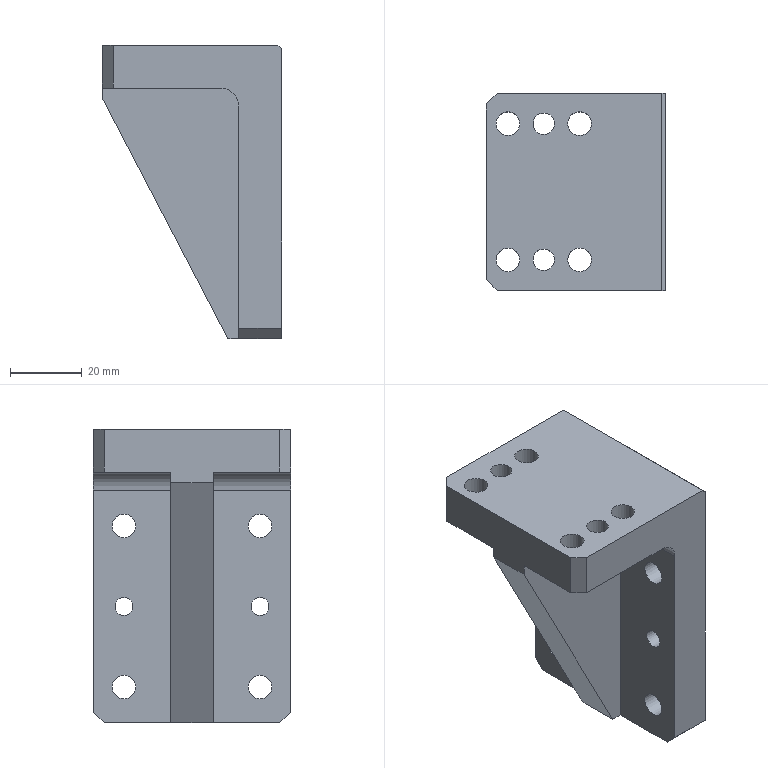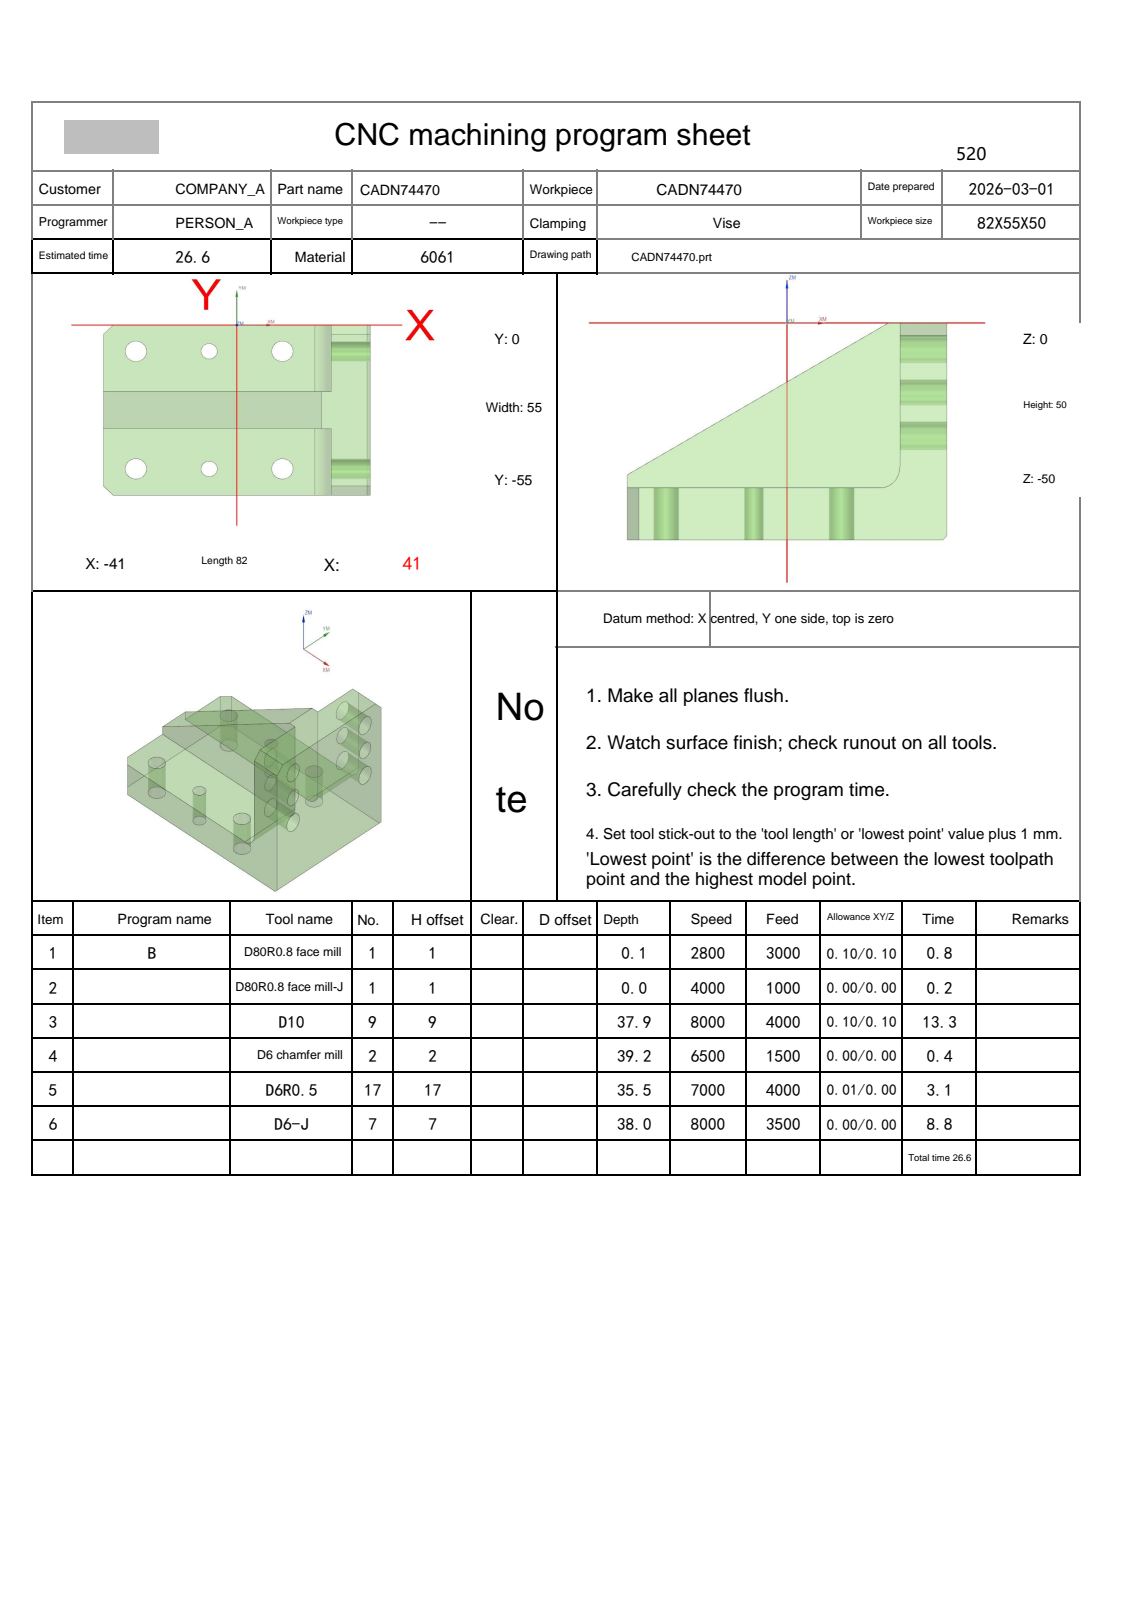NC program | NX | posted by the shop | part box 50 x 55 x 82 mm
Lines 110 to 1264 of 26562:
N3 T09 M06
(D10  D=10. R=0. H=09 ce=0.10 di=0.10)
G00 G90 G54 X-4.625 Y-69.5 M03 S8000
G43 H09 Z14.5
M08
Z.701
G01 Z-.499 F4000.
Y-62.08
G03 X-11.625 Y-55.08 I-7. J0.0
G01 X-38.
X-38.057 Y-55.057
X-41.057 Y-52.057
X-41.08 Y-52.
Y-38.676
G02 X-43.769 Y-37.838 I.201 J5.375
X-44. Y-37.666 I3.208 J4.548
G01 Y-17.36
G02 X-41.08 Y-16.324 I3.134 J-4.201
G01 Y-3.
X-41.057 Y-2.943
X-38.057 Y.057
X-38. Y.08
X23.059
X23.282 Y.077
X23.515 Y.018
X23.821 Y.019
X23.868 Y.695
X23.967 Y1.122
X24.072 Y1.563
X24.462 Y2.465
G02 X24.822 Y3. I4.707 J-2.781
G01 X25.488
G02 X29. Y4.04 I3.533 J-5.481
G01 X40.92
Y3.
X41.
Y4.04
X41.006
X41.002 Y3.
X41.08
Y2.64
X41.001
X41. Y2.641
X40.999 Y2.64
X40.92 Y2.641
X39.52 Y2.64
X29.
G03 X23.923 Y-1.998 I.021 J-5.121
G01 X23.866 Y-2.316
X23.844 Y-2.498
X23.82 Y-3.047
Y-3.243
X23.821 Y-3.438
X23.822 Y-16.544
G03 X19.829 Y-21.5 I1.102 J-4.974
G01 X19.83 Y-33.52
G03 X23.823 Y-38.456 I5.095 J.038
G01 X23.821 Y-51.562
X23.822 Y-52.069
X23.845 Y-52.508
X23.867 Y-52.688
X23.923 Y-53.002
G03 X29. Y-57.64 I5.098 J.483
G01 X39.52
X40.92
X40.999
X41. Y-57.641
X41.001 Y-57.64
X41.08
Y-58.
X41.002
X41.006 Y-59.04
X41.
Y-58.
X40.92
Y-59.04
X28.994
G02 X25.488 Y-58. I.026 J6.521
G01 X24.805
G02 X23.82 Y-55.019 I4.169 J3.032
G01 X23.515 Y-55.018
X23.398 Y-55.048
X23.262 Y-55.08
X23.024
X19.511
X19.314 Y-55.078
X18.624 Y-55.08
X-8.61
G02 X-9.423 Y-54.662 I0.0 J1.
G01 X-13.826 Y-48.498
G03 X-14.639 Y-48.08 I-.813 J-.582
G01 X-33.082
G02 X-34.08 Y-47.082 I.002 J1.
G01 Y-38.676
G03 X-36.636 Y-33.267 I-7. J0.0
G02 X-37. Y-32.498 I.636 J.771
G01 Y-22.502
G02 X-36.636 Y-21.733 I1. J-.002
G03 X-34.08 Y-16.324 I-4.444 J5.409
G01 Y-7.918
G02 X-33.082 Y-6.92 I1. J-.002
G01 X15.824
G02 X16.822 Y-7.918 I-.002 J-1.
G01 Y-12.106
G02 X16.518 Y-12.822 I-1. J.002
G03 X12.829 Y-21.487 I8.406 J-8.696
G01 Y-33.525
G03 X16.519 Y-42.179 I12.095 J.043
G02 X16.823 Y-42.895 I-.696 J-.718
G01 X16.822 Y-47.082
G02 X15.824 Y-48.08 I-1. J.002
G01 X-8.61
G02 X-9.423 Y-47.662 I0.0 J1.
G01 X-13.826 Y-41.498
G03 X-14.639 Y-41.08 I-.814 J-.582
G01 X-26.082
G02 X-27.08 Y-40.082 I.002 J1.
G01 Y-38.676
G03 X-29.807 Y-30.375 I-14. J0.0
G02 X-30. Y-29.786 I.807 J.591
G01 Y-25.214
G02 X-29.807 Y-24.625 I1. J-.002
G03 X-27.08 Y-16.324 I-11.273 J8.301
G01 Y-14.918
G02 X-26.082 Y-13.92 I1. J-.002
G01 X5.946
G02 X6.943 Y-14.92 I-.002 J-1.
X6.889 Y-15.247 I-1. J0.0
G03 X5.829 Y-21.479 I18.035 J-6.272
G01 Y-33.525
G03 X6.889 Y-39.754 I19.095 J.043
G02 X6.944 Y-40.08 I-.945 J-.326
X5.946 Y-41.08 I-1. J0.0
G01 X-8.61
G02 X-9.424 Y-40.662 I0.0 J1.
G01 X-13.826 Y-34.499
G03 X-14.639 Y-34.08 I-.814 J-.581
G01 X-19.806
G02 X-20.77 Y-33.337 I.002 J1.
G03 X-22.868 Y-28.22 I-20.31 J-5.339
G02 X-23. Y-27.726 I.868 J.496
G01 Y-27.274
G02 X-22.868 Y-26.781 I1. J-.002
G03 X-20.77 Y-21.663 I-18.212 J10.456
G02 X-19.806 Y-20.92 I.967 J-.257
G01 X-2.168
G02 X-1.171 Y-21.918 I-.002 J-1.
G01 Y-33.082
G02 X-2.168 Y-34.08 I-1. J.002
G01 X-8.961
G02 X-9.667 Y-33.787 I0.0 J1.
G01 X-13.582 Y-29.873
G03 X-14.289 Y-29.58 I-.707 J-.707
G01 X-16.581
G02 X-17.502 Y-28.963 I.003 J1.
G03 X-17.96 Y-27.92 I-23.578 J-9.713
G02 X-18.052 Y-27.5 I.908 J.419
X-17.96 Y-27.081 I1. J0.0
G03 X-17.502 Y-26.037 I-23.12 J10.757
G02 X-16.581 Y-25.42 I.924 J-.383
G01 X-6.668
G02 X-5.671 Y-26.418 I-.003 J-1.
G01 Y-28.583
G02 X-6.668 Y-29.58 I-1. J.003
G01 X-11.625
X-12.125
G03 X-19.125 Y-36.58 I0.0 J-7.
G01 Z.701
G00 Z3.
G01 X-4.625 Y-69.5 F6000.
G00 Z.203
G01 Z-.997 F4000.
Y-62.08
G03 X-11.625 Y-55.08 I-7. J0.0
G01 X-38.
X-38.057 Y-55.057
X-41.057 Y-52.057
X-41.08 Y-52.
Y-38.676
G02 X-43.769 Y-37.838 I.201 J5.375
X-46.126 Y-33.306 I3.208 J4.548
G01 X-46.121 Y-21.492
X-46.05 Y-20.789
G02 X-41.08 Y-16.324 I5.184 J-.772
G01 Y-3.
X-41.057 Y-2.943
X-38.057 Y.057
X-38. Y.08
X23.059
X23.282 Y.077
X23.515 Y.018
X23.821 Y.019
X23.868 Y.694
X24.072 Y1.563
X24.462 Y2.465
G02 X29.169 Y5.152 I4.707 J-2.781
G01 X29.267 Y5.151
X41.
X41.085 Y5.156
X41.08 Y5.071
Y3.139
X41.
X40.92
X29.
G03 X23.898 Y-1.984 I.021 J-5.122
G01 X23.9 Y-2.114
X23.866 Y-2.316
X23.844 Y-2.498
X23.82 Y-3.047
Y-3.243
X23.821 Y-3.438
X23.822 Y-16.408
G03 X18.875 Y-21.5 I.239 J-5.181
G01 Y-33.5
G03 X23.823 Y-38.592 I5.186 J.089
G01 X23.821 Y-51.562
X23.822 Y-52.069
X23.845 Y-52.508
X23.867 Y-52.688
X23.9 Y-52.887
Y-52.997
Y-53.018
G03 X29. Y-58.139 I5.121 J0.0
G01 X40.92
X41.
X41.08
Y-60.071
X41.085 Y-60.156
X41. Y-60.151
X29.262
X28.363 Y-60.092
X27.47 Y-59.899
G02 X23.82 Y-55.019 I1.505 J4.931
G01 X23.515 Y-55.018
X23.262 Y-55.08
X19.511
X19.314 Y-55.078
X18.624 Y-55.08
X-8.61
G02 X-9.423 Y-54.662 I0.0 J1.
G01 X-13.826 Y-48.498
G03 X-14.639 Y-48.08 I-.814 J-.582
G01 X-33.081
G02 X-34.08 Y-47.081 I.001 J1.
G01 Y-38.676
G03 X-38.496 Y-32.17 I-7. J0.0
G02 X-39.125 Y-31.243 I.371 J.929
G01 X-39.123 Y-23.756
G02 X-38.494 Y-22.829 I1. J-.002
G03 X-34.08 Y-16.324 I-2.586 J6.505
G01 Y-7.919
G02 X-33.081 Y-6.92 I1. J-.001
G01 X15.823
G02 X16.822 Y-7.919 I-.001 J-1.
G01 Y-11.294
G02 X16.448 Y-12.073 I-1. J.001
G03 X11.875 Y-21.44 I7.613 J-9.516
G01 X11.876 Y-33.62
G03 X16.448 Y-42.928 I12.185 J.209
G02 X16.823 Y-43.707 I-.626 J-.78
G01 X16.822 Y-47.082
G02 X15.824 Y-48.08 I-1. J.002
G01 X-8.61
G02 X-9.423 Y-47.662 I0.0 J1.
G01 X-13.826 Y-41.498
G03 X-14.639 Y-41.08 I-.814 J-.582
G01 X-26.082
G02 X-27.08 Y-40.082 I.002 J1.
G01 Y-38.676
G03 X-31.744 Y-28.244 I-14. J0.0
G02 X-32.075 Y-27.5 I.668 J.744
X-31.744 Y-26.756 I1. J0.0
G03 X-27.08 Y-16.324 I-9.336 J10.432
G01 Y-14.918
G02 X-26.082 Y-13.92 I1. J-.002
G01 X5.009
G02 X6.007 Y-14.92 I-.002 J-1.
X5.952 Y-15.249 I-1. J0.0
G03 X4.875 Y-21.354 I18.109 J-6.34
G01 X4.877 Y-33.74
G03 X5.952 Y-39.751 I19.184 J.329
G02 X6.007 Y-40.08 I-.944 J-.329
X5.009 Y-41.08 I-1. J0.0
G01 X-8.61
G02 X-9.423 Y-40.662 I0.0 J1.
G01 X-13.826 Y-34.499
G03 X-14.639 Y-34.08 I-.814 J-.581
G01 X-19.806
G02 X-20.77 Y-33.336 I.002 J1.
G03 X-22.993 Y-28.006 I-20.31 J-5.34
G02 X-23.13 Y-27.5 I.862 J.506
X-22.993 Y-26.994 I1. J0.0
G03 X-20.77 Y-21.664 I-18.087 J10.67
G02 X-19.806 Y-20.92 I.967 J-.256
G01 X-3.123
G02 X-2.125 Y-21.918 I-.002 J-1.
G01 X-2.123 Y-33.082
G02 X-3.121 Y-34.08 I-1. J.002
G01 X-8.961
G02 X-9.667 Y-33.787 I0.0 J1.
G01 X-13.582 Y-29.873
G03 X-14.289 Y-29.58 I-.707 J-.707
G01 X-16.581
G02 X-17.502 Y-28.963 I.002 J1.
G03 X-17.96 Y-27.92 I-23.578 J-9.713
G02 X-18.052 Y-27.5 I.908 J.42
X-17.96 Y-27.08 I1. J0.0
G03 X-17.502 Y-26.037 I-23.12 J10.756
G02 X-16.581 Y-25.42 I.924 J-.383
G01 X-7.622
G02 X-6.624 Y-26.418 I-.002 J-1.
G01 Y-28.582
G02 X-7.622 Y-29.58 I-1. J.002
G01 X-11.625
X-12.125
G03 X-19.125 Y-36.58 I0.0 J-7.
G01 Z.203
G00 Z3.
G01 X-4.625 Y-69.5 F6000.
G00 Z-.296
G01 Z-1.496 F4000.
Y-62.08
G03 X-11.625 Y-55.08 I-7. J0.0
G01 X-38.
X-38.057 Y-55.057
X-41.057 Y-52.057
X-41.08 Y-52.
Y-38.676
G02 X-43.769 Y-37.838 I.201 J5.375
X-46.126 Y-33.306 I3.208 J4.548
G01 X-46.121 Y-21.492
X-46.05 Y-20.789
G02 X-41.08 Y-16.324 I5.184 J-.772
G01 Y-3.
X-41.057 Y-2.943
X-38.057 Y.057
X-38. Y.08
X23.059
X23.282 Y.077
X23.515 Y.018
X23.821 Y.019
X23.868 Y.694
X24.072 Y1.563
X24.462 Y2.465
G02 X29.169 Y5.152 I4.707 J-2.781
G01 X29.267 Y5.151
X41.
X41.085 Y5.156
X41.08 Y5.071
Y3.637
X41.
X40.92
X29.
G03 X23.9 Y-1.504 I.046 J-5.146
G01 Y-2.114
X23.866 Y-2.316
X23.844 Y-2.498
X23.82 Y-3.047
Y-3.243
X23.821 Y-3.438
X23.822 Y-16.4
X23.136
X23.078
G03 X17.92 Y-21.5 I0.0 J-5.158
G01 Y-33.5
G03 X23.078 Y-38.6 I5.158 J.058
G01 X23.136
X23.823
X23.821 Y-51.562
X23.822 Y-52.069
X23.845 Y-52.508
X23.867 Y-52.688
X23.9 Y-52.887
Y-53.496
G03 X29. Y-58.637 I5.146 J.005
G01 X40.92
X41.
X41.08
Y-60.071
X41.085 Y-60.156
X41. Y-60.151
X29.262
X28.363 Y-60.092
X27.47 Y-59.899
G02 X23.82 Y-55.019 I1.505 J4.931
G01 X23.515 Y-55.018
X23.262 Y-55.08
X19.511
X19.314 Y-55.078
X18.624 Y-55.08
X-8.61
G02 X-9.423 Y-54.662 I0.0 J1.
G01 X-13.826 Y-48.498
G03 X-14.639 Y-48.08 I-.814 J-.582
G01 X-33.082
G02 X-34.08 Y-47.082 I.002 J1.
G01 Y-38.676
G03 X-38.496 Y-32.17 I-7. J0.0
G02 X-39.125 Y-31.243 I.371 J.929
G01 X-39.123 Y-23.755
G02 X-38.494 Y-22.829 I1. J-.002
G03 X-34.08 Y-16.324 I-2.586 J6.505
G01 Y-7.918
G02 X-33.082 Y-6.92 I1. J-.002
G01 X15.823
G02 X16.822 Y-7.919 I-.002 J-1.
G01 Y-10.583
G02 X16.375 Y-11.415 I-1. J.002
G03 X10.92 Y-21.461 I6.704 J-10.143
G01 Y-33.539
G03 X16.375 Y-43.586 I12.158 J.097
G02 X16.823 Y-44.418 I-.553 J-.833
G01 X16.822 Y-47.082
G02 X15.824 Y-48.08 I-1. J.002
G01 X-8.61
G02 X-9.423 Y-47.662 I0.0 J1.
G01 X-13.826 Y-41.498
G03 X-14.639 Y-41.08 I-.814 J-.582
G01 X-26.082
G02 X-27.08 Y-40.082 I.002 J1.
G01 Y-38.676
G03 X-31.744 Y-28.244 I-14. J0.0
G02 X-32.075 Y-27.5 I.668 J.744
X-31.744 Y-26.756 I1. J0.0
G03 X-27.08 Y-16.324 I-9.336 J10.432
G01 Y-14.918
G02 X-26.082 Y-13.92 I1. J-.002
G01 X4.046
G02 X5.044 Y-14.92 I-.002 J-1.
X4.989 Y-15.248 I-1. J0.0
G03 X3.92 Y-21.433 I18.089 J-6.31
G01 Y-33.567
G03 X4.989 Y-39.753 I19.158 J.125
G02 X5.044 Y-40.08 I-.945 J-.327
X4.046 Y-41.08 I-1. J0.0
G01 X-8.61
G02 X-9.424 Y-40.662 I0.0 J1.
G01 X-13.826 Y-34.499
G03 X-14.639 Y-34.08 I-.814 J-.581
G01 X-19.806
G02 X-20.77 Y-33.337 I.002 J1.
G03 X-22.993 Y-28.006 I-20.31 J-5.34
G02 X-23.13 Y-27.5 I.862 J.506
X-22.993 Y-26.994 I1. J0.0
G03 X-20.77 Y-21.664 I-18.087 J10.67
G02 X-19.806 Y-20.92 I.967 J-.257
G01 X-4.078
G02 X-3.08 Y-21.918 I-.002 J-1.
G01 Y-33.082
G02 X-4.078 Y-34.08 I-1. J.002
G01 X-8.961
G02 X-9.667 Y-33.787 I0.0 J1.
G01 X-13.582 Y-29.873
G03 X-14.289 Y-29.58 I-.707 J-.707
G01 X-16.581
G02 X-17.502 Y-28.963 I.002 J1.
G03 X-17.96 Y-27.92 I-23.578 J-9.713
G02 X-18.052 Y-27.5 I.908 J.42
X-17.96 Y-27.081 I1. J0.0
G03 X-17.502 Y-26.037 I-23.12 J10.756
G02 X-16.581 Y-25.42 I.924 J-.383
G01 X-8.577
G02 X-7.58 Y-26.418 I-.002 J-1.
G01 Y-28.582
G02 X-8.577 Y-29.58 I-1. J.002
G01 X-11.625
X-12.125
G03 X-19.125 Y-36.58 I0.0 J-7.
G01 Z-.296
G00 Z3.
G01 X-4.625 Y-69.5 F6000.
G00 Z-.795
G01 Z-1.995 F4000.
Y-62.08
G03 X-11.625 Y-55.08 I-7. J0.0
G01 X-38.
X-38.057 Y-55.057
X-41.057 Y-52.057
X-41.08 Y-52.
Y-38.676
G02 X-43.769 Y-37.838 I.201 J5.375
X-46.126 Y-33.306 I3.208 J4.548
G01 X-46.121 Y-21.492
X-46.05 Y-20.789
G02 X-41.08 Y-16.324 I5.184 J-.772
G01 Y-3.
X-41.057 Y-2.943
X-38.057 Y.057
X-38. Y.08
X23.059
X23.282 Y.077
X23.515 Y.018
X23.821 Y.019
X23.868 Y.694
X24.072 Y1.563
X24.462 Y2.465
G02 X29.169 Y5.152 I4.707 J-2.781
G01 X29.267 Y5.151
X41.
X41.085 Y5.156
X41.08 Y5.071
Y4.136
X41.
X40.998
X40.92
X29.
G03 X23.9 Y-.985 I.021 J-5.121
G01 Y-1.005
Y-2.114
X23.866 Y-2.316
X23.844 Y-2.498
X23.82 Y-3.047
Y-3.243
X23.821 Y-3.438
X23.822 Y-16.4
X22.181
X22.123
G03 X16.966 Y-21.5 I0.0 J-5.158
G01 Y-33.5
G03 X22.123 Y-38.6 I5.158 J.058
G01 X22.181
X23.823
X23.821 Y-51.562
X23.822 Y-52.069
X23.845 Y-52.508
X23.867 Y-52.688
X23.9 Y-52.887
Y-53.995
Y-54.015
G03 X29. Y-59.136 I5.121 J0.0
G01 X40.92
X40.998
X41.
X41.08
Y-60.071
X41.085 Y-60.156
X41. Y-60.151
X29.262
X28.363 Y-60.092
X27.47 Y-59.899
G02 X23.82 Y-55.019 I1.505 J4.931
G01 X23.515 Y-55.018
X23.262 Y-55.08
X19.511
X19.314 Y-55.078
X18.624 Y-55.08
X-8.61
G02 X-9.423 Y-54.662 I0.0 J1.
G01 X-13.826 Y-48.498
G03 X-14.639 Y-48.08 I-.814 J-.582
G01 X-33.082
G02 X-34.08 Y-47.082 I.002 J1.
G01 Y-38.676
G03 X-38.496 Y-32.17 I-7. J0.0
G02 X-39.125 Y-31.243 I.371 J.929
G01 X-39.123 Y-23.755
G02 X-38.494 Y-22.829 I1. J-.002
G03 X-34.08 Y-16.324 I-2.586 J6.505
G01 Y-7.918
G02 X-33.082 Y-6.92 I1. J-.002
G01 X15.823
G02 X16.822 Y-7.918 I-.002 J-1.
G01 Y-10.009
G02 X16.302 Y-10.884 I-1. J.002
G03 X9.966 Y-21.461 I5.821 J-10.674
G01 Y-33.539
G03 X16.303 Y-44.117 I12.158 J.097
G02 X16.822 Y-44.992 I-.48 J-.877
G01 Y-47.082
G02 X15.824 Y-48.08 I-1. J.002
G01 X-8.61
G02 X-9.423 Y-47.662 I0.0 J1.
G01 X-13.826 Y-41.498
G03 X-14.639 Y-41.08 I-.814 J-.582
G01 X-26.082
G02 X-27.08 Y-40.082 I.002 J1.
G01 Y-38.676
G03 X-31.744 Y-28.244 I-14. J0.0
G02 X-32.075 Y-27.5 I.669 J.744
X-31.744 Y-26.756 I1. J0.0
G03 X-27.08 Y-16.324 I-9.336 J10.432
G01 Y-14.918
G02 X-26.082 Y-13.92 I1. J-.002
G01 X3.092
G02 X4.089 Y-14.92 I-.002 J-1.
X4.034 Y-15.248 I-1. J0.0
G03 X2.966 Y-21.404 I18.089 J-6.31
G01 Y-33.595
G03 X4.034 Y-39.753 I19.158 J.153
G02 X4.089 Y-40.08 I-.945 J-.327
X3.092 Y-41.08 I-1. J0.0
G01 X-8.61
G02 X-9.424 Y-40.662 I0.0 J1.
G01 X-13.826 Y-34.499
G03 X-14.639 Y-34.08 I-.814 J-.581
G01 X-19.806
G02 X-20.77 Y-33.337 I.002 J1.
G03 X-22.993 Y-28.006 I-20.31 J-5.34
G02 X-23.13 Y-27.5 I.863 J.506
X-22.993 Y-26.994 I1. J0.0
G03 X-20.77 Y-21.663 I-18.087 J10.67
G02 X-19.806 Y-20.92 I.967 J-.257
G01 X-5.032
G02 X-4.034 Y-21.918 I-.002 J-1.
G01 Y-33.082
G02 X-5.032 Y-34.08 I-1. J.002
G01 X-8.961
G02 X-9.667 Y-33.787 I0.0 J1.
G01 X-13.582 Y-29.873
G03 X-14.289 Y-29.58 I-.707 J-.707
G01 X-16.581
G02 X-17.502 Y-28.963 I.003 J1.
G03 X-17.96 Y-27.92 I-23.578 J-9.713
G02 X-18.052 Y-27.5 I.908 J.42
X-17.96 Y-27.081 I1. J0.0
G03 X-17.502 Y-26.037 I-23.12 J10.757
G02 X-16.581 Y-25.42 I.924 J-.383
G01 X-9.532
G02 X-8.534 Y-26.418 I-.003 J-1.
G01 Y-28.583
G02 X-9.532 Y-29.58 I-1. J.003
G01 X-11.625
X-12.125
G03 X-19.125 Y-36.58 I0.0 J-7.
G01 Z-.795
G00 Z3.
G01 X-4.625 Y-69.5 F6000.
G00 Z-1.293
G01 Z-2.493 F4000.
Y-62.08
G03 X-11.625 Y-55.08 I-7. J0.0
G01 X-38.
X-38.057 Y-55.057
X-41.057 Y-52.057
X-41.08 Y-52.
Y-38.676
G02 X-43.769 Y-37.838 I.201 J5.375
X-46.126 Y-33.306 I3.208 J4.548
G01 X-46.121 Y-21.492
X-46.05 Y-20.789
G02 X-41.08 Y-16.324 I5.184 J-.772
G01 Y-3.
X-41.057 Y-2.943
X-38.057 Y.057
X-38. Y.08
X23.059
X23.282 Y.077
X23.515 Y.018
X23.821 Y.019
X23.868 Y.694
X24.072 Y1.563
X24.462 Y2.465
G02 X29.169 Y5.152 I4.707 J-2.781
G01 X29.267 Y5.151
X41.
X41.085 Y5.156
X41.08 Y5.071
Y4.635
X41.
X40.989
X40.92
X29.
G03 X23.9 Y-.507 I.052 J-5.151
G01 Y-2.114
X23.866 Y-2.316
X23.844 Y-2.498
X23.82 Y-3.047
Y-3.243
X23.821 Y-3.438
X23.822 Y-16.4
X21.227
X21.169
G03 X16.011 Y-21.5 I0.0 J-5.158
G01 Y-33.5
G03 X21.169 Y-38.6 I5.158 J.058
G01 X21.227
X23.823
X23.821 Y-51.562
X23.822 Y-52.069
X23.845 Y-52.508
X23.867 Y-52.688
X23.9 Y-52.887
Y-54.493
G03 X29. Y-59.635 I5.151 J.01
G01 X40.92
X40.989
X41.
X41.08
Y-60.071
X41.085 Y-60.156
X41. Y-60.151
X29.262
X28.363 Y-60.092
X27.47 Y-59.899
G02 X23.82 Y-55.019 I1.505 J4.931
G01 X23.515 Y-55.018
X23.262 Y-55.08
X19.511
X19.314 Y-55.078
X18.624 Y-55.08
X-8.61
G02 X-9.423 Y-54.662 I0.0 J1.
G01 X-13.826 Y-48.498
G03 X-14.639 Y-48.08 I-.813 J-.582
G01 X-33.082
G02 X-34.08 Y-47.082 I.002 J1.
G01 Y-38.676
G03 X-38.497 Y-32.17 I-7. J0.0
G02 X-39.125 Y-31.243 I.371 J.929
G01 X-39.123 Y-23.755
G02 X-38.494 Y-22.829 I1. J-.002
G03 X-34.08 Y-16.324 I-2.586 J6.505
G01 Y-7.918
G02 X-33.082 Y-6.92 I1. J-.002
G01 X15.824
G02 X16.822 Y-7.918 I-.002 J-1.
G01 Y-9.537
G02 X16.23 Y-10.448 I-1. J.002
G03 X9.011 Y-21.461 I4.939 J-11.11
G01 Y-33.579
G03 X16.23 Y-44.552 I12.158 J.137
G02 X16.822 Y-45.463 I-.408 J-.913
G01 Y-47.082
G02 X15.824 Y-48.08 I-1. J.002
G01 X-8.61
G02 X-9.423 Y-47.662 I0.0 J1.
G01 X-13.826 Y-41.498
G03 X-14.639 Y-41.08 I-.814 J-.582
G01 X-26.082
G02 X-27.08 Y-40.082 I.002 J1.
G01 Y-38.676
G03 X-31.744 Y-28.244 I-14. J0.0
G02 X-32.075 Y-27.5 I.669 J.744
X-31.744 Y-26.757 I1. J0.0
G03 X-27.08 Y-16.324 I-9.336 J10.432
G01 Y-14.918
G02 X-26.082 Y-13.92 I1. J-.002
G01 X2.137
G02 X3.135 Y-14.92 I-.002 J-1.
X3.08 Y-15.247 I-1. J0.0
G03 X2.011 Y-21.404 I18.089 J-6.311
G01 X2.012 Y-33.657
G03 X3.08 Y-39.753 I19.157 J.215
G02 X3.135 Y-40.08 I-.945 J-.327
X2.137 Y-41.08 I-1. J0.0
G01 X-8.61
G02 X-9.424 Y-40.662 I0.0 J1.
G01 X-13.826 Y-34.499
G03 X-14.639 Y-34.08 I-.814 J-.581
G01 X-19.806
G02 X-20.77 Y-33.337 I.003 J1.
G03 X-22.993 Y-28.006 I-20.31 J-5.339
G02 X-23.13 Y-27.5 I.863 J.506
X-22.993 Y-26.994 I1. J0.0
G03 X-20.77 Y-21.663 I-18.087 J10.67
G02 X-19.806 Y-20.92 I.966 J-.257
G01 X-5.986
G02 X-4.989 Y-21.918 I-.003 J-1.
G01 X-4.988 Y-33.082
G02 X-5.986 Y-34.08 I-1. J.002
G01 X-8.961
G02 X-9.667 Y-33.787 I0.0 J1.
G01 X-13.582 Y-29.873
G03 X-14.289 Y-29.58 I-.707 J-.707
G01 X-16.581
G02 X-17.502 Y-28.963 I.003 J1.
G03 X-17.96 Y-27.92 I-23.578 J-9.713
G02 X-18.052 Y-27.5 I.908 J.419
X-17.96 Y-27.081 I1. J0.0
G03 X-17.502 Y-26.037 I-23.12 J10.757
G02 X-16.581 Y-25.42 I.924 J-.383
G01 X-10.486
G02 X-9.489 Y-26.417 I-.003 J-1.
G01 X-9.488 Y-28.583
G02 X-10.486 Y-29.58 I-1. J.003
G01 X-11.625
X-12.125
G03 X-19.125 Y-36.58 I0.0 J-7.
G01 Z-1.293
G00 Z3.
G01 X-4.625 Y-69.5 F6000.
G00 Z-1.792
G01 Z-2.992 F4000.
Y-62.08
G03 X-11.625 Y-55.08 I-7. J0.0
G01 X-38.
X-38.057 Y-55.057
X-41.057 Y-52.057
X-41.08 Y-52.
Y-38.676
G02 X-43.769 Y-37.838 I.201 J5.375
X-44. Y-37.666 I3.208 J4.548
G01 Y-17.36
G02 X-41.08 Y-16.324 I3.134 J-4.201
G01 Y-3.
X-41.057 Y-2.943
X-38.057 Y.057
X-38. Y.08
X22.5
X23.059
X23.282 Y.077
X23.515 Y.018
X23.821 Y.019
X23.866 Y.678
X23.933 Y.672
X23.9 Y.658
Y-2.114
X23.866 Y-2.316
X23.844 Y-2.498
X23.82 Y-3.047
Y-3.243
X23.821 Y-3.438
X23.822 Y-16.4
X20.272
X20.214
G03 X15.056 Y-21.5 I0.0 J-5.158
G01 Y-33.5
G03 X20.214 Y-38.6 I5.158 J.058
G01 X20.272
X23.823
Y-40.
X23.821 Y-51.562
X23.822 Y-52.069
X23.845 Y-52.508
X23.867 Y-52.688
X23.9 Y-52.887
Y-55.659
X23.938 Y-55.674
X23.869 Y-55.684
G02 X23.82 Y-55.019 I5.105 J.716
G01 X23.515 Y-55.018
X23.398 Y-55.048
X23.262 Y-55.08
X22.5
X19.511
X19.314 Y-55.078
X18.624 Y-55.08
X-8.61
G02 X-9.423 Y-54.662 I0.0 J1.
G01 X-13.826 Y-48.498
G03 X-14.639 Y-48.08 I-.813 J-.582
G01 X-33.083
G02 X-34.08 Y-47.083 I.003 J1.
G01 Y-38.676
G03 X-36.637 Y-33.267 I-7. J0.0
G02 X-37. Y-32.499 I.637 J.771
G01 Y-22.502
G02 X-36.637 Y-21.733 I1. J-.003
G03 X-34.08 Y-16.324 I-4.443 J5.409
G01 Y-7.917
G02 X-33.083 Y-6.92 I1. J-.003
G01 X15.824
G02 X16.822 Y-7.918 I-.003 J-1.
G01 Y-9.157
G02 X16.158 Y-10.096 I-1. J.002
G03 X8.056 Y-21.461 I4.056 J-11.462
G01 Y-33.539
G03 X9.222 Y-38.638 I12.158 J.098
X16.158 Y-44.904 I10.992 J5.196
G02 X16.822 Y-45.843 I-.336 J-.942
G01 Y-47.083
G02 X15.825 Y-48.08 I-1. J.003
G01 X-8.61
G02 X-9.423 Y-47.662 I0.0 J1.
G01 X-13.826 Y-41.498
G03 X-14.639 Y-41.08 I-.814 J-.582
G01 X-26.083
G02 X-27.08 Y-40.083 I.003 J1.
G01 Y-38.676
G03 X-29.807 Y-30.375 I-14. J0.0
G02 X-30. Y-29.787 I.807 J.591
G01 Y-25.214
G02 X-29.807 Y-24.626 I1. J-.003
G03 X-27.08 Y-16.324 I-11.273 J8.302
G01 Y-14.917
G02 X-26.083 Y-13.92 I1. J-.003
G01 X1.183
G02 X2.18 Y-14.92 I-.003 J-1.
X2.125 Y-15.247 I-1. J0.0
G03 X1.056 Y-21.433 I18.089 J-6.311
G01 Y-33.567
G03 X2.125 Y-39.753 I19.158 J.126
G02 X2.18 Y-40.08 I-.945 J-.327
X1.183 Y-41.08 I-1. J0.0
G01 X-8.61
G02 X-9.424 Y-40.662 I0.0 J1.
G01 X-13.826 Y-34.499
G03 X-14.639 Y-34.08 I-.814 J-.581
G01 X-19.807
G02 X-20.77 Y-33.337 I.003 J1.
G03 X-22.869 Y-28.219 I-20.31 J-5.339
G02 X-23. Y-27.727 I.869 J.495
G01 Y-27.273
G02 X-22.869 Y-26.781 I1. J-.003
G03 X-20.77 Y-21.663 I-18.211 J10.457
G02 X-19.807 Y-20.92 I.966 J-.257
G01 X-6.941
G02 X-5.944 Y-21.917 I-.003 J-1.
G01 Y-33.083
G02 X-6.941 Y-34.08 I-1. J.003
G01 X-8.961
G02 X-9.667 Y-33.787 I0.0 J1.
G01 X-13.582 Y-29.873
G03 X-14.289 Y-29.58 I-.707 J-.707
G01 X-16.582
G02 X-17.502 Y-28.964 I.003 J1.
G03 X-17.96 Y-27.919 I-23.578 J-9.712
G02 X-18.052 Y-27.5 I.908 J.419
X-17.96 Y-27.081 I1. J0.0
G03 X-17.502 Y-26.036 I-23.12 J10.757
G02 X-16.582 Y-25.42 I.923 J-.384
G01 X-11.441
G02 X-10.444 Y-26.417 I-.003 J-1.
G01 Y-28.583
G02 X-11.441 Y-29.58 I-1. J.003
G01 X-11.625
X-12.125
G03 X-19.125 Y-36.58 I0.0 J-7.
G01 Z-1.792
G00 Z3.
G01 X-4.625 Y-69.5 F6000.
G00 Z-2.291
G01 Z-3.491 F4000.
Y-62.08
G03 X-11.625 Y-55.08 I-7. J0.0
G01 X-38.
X-38.057 Y-55.057
X-41.057 Y-52.057
X-41.08 Y-52.
Y-38.676
G02 X-43.769 Y-37.838 I.201 J5.375
X-44. Y-37.666 I3.208 J4.548
G01 Y-17.36
G02 X-41.08 Y-16.324 I3.134 J-4.201
G01 Y-3.
X-41.057 Y-2.943
X-38.057 Y.057
X-38. Y.08
X23.059
X23.282 Y.077
X23.515 Y.018
X23.821 Y.019
X23.899 Y.01
X23.9 Y-2.114
X23.866 Y-2.316
X23.844 Y-2.498
X23.82 Y-3.047
Y-3.243
X23.821 Y-3.438
X23.822 Y-16.4
X19.318
X19.266
G03 X14.102 Y-21.5 I0.0 J-5.165
G01 Y-33.5
G03 X19.266 Y-38.6 I5.164 J.064
G01 X19.318
X23.823
X23.821 Y-51.562
X23.822 Y-52.069
X23.845 Y-52.508
X23.867 Y-52.688
X23.9 Y-52.887
Y-55.01
X23.82 Y-55.019
X23.515 Y-55.018
X23.262 Y-55.08
X19.511
X19.314 Y-55.078
X18.624 Y-55.08
X-8.61
G02 X-9.423 Y-54.662 I0.0 J1.
G01 X-13.826 Y-48.498
G03 X-14.639 Y-48.08 I-.814 J-.582
G01 X-33.083
G02 X-34.08 Y-47.083 I.003 J1.
G01 Y-38.676
G03 X-36.637 Y-33.267 I-7. J0.0
G02 X-37. Y-32.499 I.637 J.771
G01 Y-22.502
G02 X-36.637 Y-21.733 I1. J-.003
G03 X-34.08 Y-16.324 I-4.443 J5.409
G01 Y-7.917
G02 X-33.083 Y-6.92 I1. J-.003
G01 X15.824
G02 X16.822 Y-7.918 I-.003 J-1.
G01 Y-8.861
G02 X16.086 Y-9.823 I-1. J.003
G03 X8.989 Y-15.055 I3.18 J-11.742
X7.102 Y-21.456 I10.277 J-6.509
G01 Y-33.544
G03 X16.086 Y-45.177 I12.164 J.108
G02 X16.822 Y-46.139 I-.264 J-.965
G01 Y-47.083
G02 X15.825 Y-48.08 I-1. J.003
G01 X-8.61
G02 X-9.423 Y-47.662 I0.0 J1.
G01 X-13.826 Y-41.498
G03 X-14.639 Y-41.08 I-.814 J-.582
G01 X-26.083
G02 X-27.08 Y-40.083 I.003 J1.
G01 Y-38.676
G03 X-29.807 Y-30.374 I-14. J0.0
G02 X-30. Y-29.787 I.807 J.591
G01 Y-25.214
G02 X-29.807 Y-24.626 I1. J-.003
G03 X-27.08 Y-16.324 I-11.273 J8.302
G01 Y-14.917
G02 X-26.083 Y-13.92 I1. J-.003
G01 X.23
G02 X1.227 Y-14.92 I-.003 J-1.
X1.172 Y-15.247 I-1. J0.0
G03 X.102 Y-21.425 I18.093 J-6.317
G01 Y-33.575
G03 X1.172 Y-39.753 I19.164 J.139
G02 X1.227 Y-40.08 I-.945 J-.327
X.23 Y-41.08 I-1. J0.0
G01 X-8.61
G02 X-9.424 Y-40.662 I0.0 J1.
G01 X-13.826 Y-34.499
G03 X-14.639 Y-34.08 I-.814 J-.581
G01 X-19.807
G02 X-20.77 Y-33.337 I.003 J1.
G03 X-22.869 Y-28.219 I-20.31 J-5.339
G02 X-23. Y-27.727 I.869 J.495
G01 Y-27.273
G02 X-22.869 Y-26.781 I1. J-.003
G03 X-20.77 Y-21.663 I-18.211 J10.457
G02 X-19.807 Y-20.92 I.966 J-.257
G01 X-7.895
G02 X-6.898 Y-21.917 I-.003 J-1.
G01 Y-33.083
G02 X-7.895 Y-34.08 I-1. J.003
G01 X-8.975
G02 X-9.629 Y-33.836 I0.0 J1.
G01 X-14.254 Y-29.824
G03 X-14.909 Y-29.58 I-.655 J-.756
G01 X-16.582
G02 X-17.502 Y-28.964 I.003 J1.
G03 X-17.96 Y-27.919 I-23.578 J-9.712
G02 X-18.052 Y-27.5 I.908 J.419
X-17.96 Y-27.081 I1. J0.0
G03 X-17.502 Y-26.036 I-23.12 J10.757
G02 X-16.582 Y-25.42 I.923 J-.384
G01 X-12.395
G02 X-11.398 Y-26.417 I-.003 J-1.
G01 Y-28.583
G02 X-12.259 Y-29.57 I-1. J.003
G01 X-12.395 Y-29.58
X-12.759
G03 X-19.759 Y-36.58 I0.0 J-7.
G01 Z-2.291
G00 Z3.
G01 X-4.625 Y-69.5 F6000.
G00 Z-2.789
G01 Z-3.989 F4000.
Y-62.08
G03 X-11.625 Y-55.08 I-7. J0.0
G01 X-38.
X-38.057 Y-55.057
X-41.057 Y-52.057
X-41.08 Y-52.
Y-38.676
G02 X-43.769 Y-37.838 I.201 J5.375
X-44. Y-37.666 I3.208 J4.548
G01 Y-17.36
G02 X-41.08 Y-16.324 I3.134 J-4.201
G01 Y-3.
X-41.057 Y-2.943
X-38.057 Y.057
X-38. Y.08
X23.059
X23.282 Y.077
X23.515 Y.018
X23.821 Y.019
X23.899 Y.01
X23.9 Y-2.114
X23.866 Y-2.316
X23.844 Y-2.498
X23.82 Y-3.047
Y-3.243
X23.821 Y-3.438
X23.822 Y-15.
Y-16.4
X22.422
X18.363
X18.315
G03 X13.147 Y-21.5 I0.0 J-5.168
G01 Y-33.5
G03 X18.315 Y-38.6 I5.167 J.068
G01 X18.363
X23.823
X23.821 Y-51.562
X23.822 Y-52.069
X23.845 Y-52.508
X23.867 Y-52.688
X23.9 Y-52.887
Y-55.01
X23.82 Y-55.019
X23.515 Y-55.018
X23.262 Y-55.08
X19.511
X19.314 Y-55.078
X18.624 Y-55.08
X-8.61
G02 X-9.423 Y-54.662 I0.0 J1.
G01 X-13.826 Y-48.498
G03 X-14.639 Y-48.08 I-.814 J-.582
G01 X-33.083
G02 X-34.08 Y-47.083 I.003 J1.
G01 Y-38.676
G03 X-36.637 Y-33.267 I-7. J0.0
G02 X-37. Y-32.499 I.637 J.771
G01 Y-22.501
G02 X-36.637 Y-21.733 I1. J-.003
G03 X-34.08 Y-16.324 I-4.443 J5.409
G01 Y-7.917
G02 X-33.083 Y-6.92 I1. J-.003
G01 X15.824
G02 X16.822 Y-7.918 I-.003 J-1.
G01 Y-8.641
G02 X16.014 Y-9.619 I-1. J.003
G03 X6.147 Y-21.454 I2.301 J-11.948
G01 X6.148 Y-33.592
G03 X16.014 Y-45.381 I12.167 J.16
G02 X16.822 Y-46.36 I-.192 J-.981
G01 Y-47.083
G02 X15.825 Y-48.08 I-1. J.003
G01 X-8.61
G02 X-9.423 Y-47.662 I0.0 J1.
G01 X-13.826 Y-41.498
G03 X-14.639 Y-41.08 I-.814 J-.582
G01 X-26.083
G02 X-27.08 Y-40.083 I.003 J1.
G01 Y-38.676
G03 X-29.807 Y-30.374 I-14. J0.0
G02 X-30. Y-29.787 I.807 J.59
G01 Y-25.213
G02 X-29.807 Y-24.626 I1. J-.003
G03 X-27.08 Y-16.324 I-11.273 J8.302
G01 Y-14.917
G02 X-26.083 Y-13.92 I1. J-.003
G01 X-.723
G02 X.274 Y-14.92 I-.003 J-1.
X.219 Y-15.247 I-1. J0.0
G03 X-.853 Y-21.422 I18.096 J-6.321
G01 X-.852 Y-33.638
G03 X.219 Y-39.753 I19.167 J.206
G02 X.274 Y-40.08 I-.945 J-.327
X-.723 Y-41.08 I-1. J0.0
G01 X-8.61
G02 X-9.424 Y-40.662 I0.0 J1.
G01 X-13.826 Y-34.499
G03 X-14.639 Y-34.08 I-.814 J-.581
G01 X-19.807
G02 X-20.77 Y-33.337 I.003 J1.